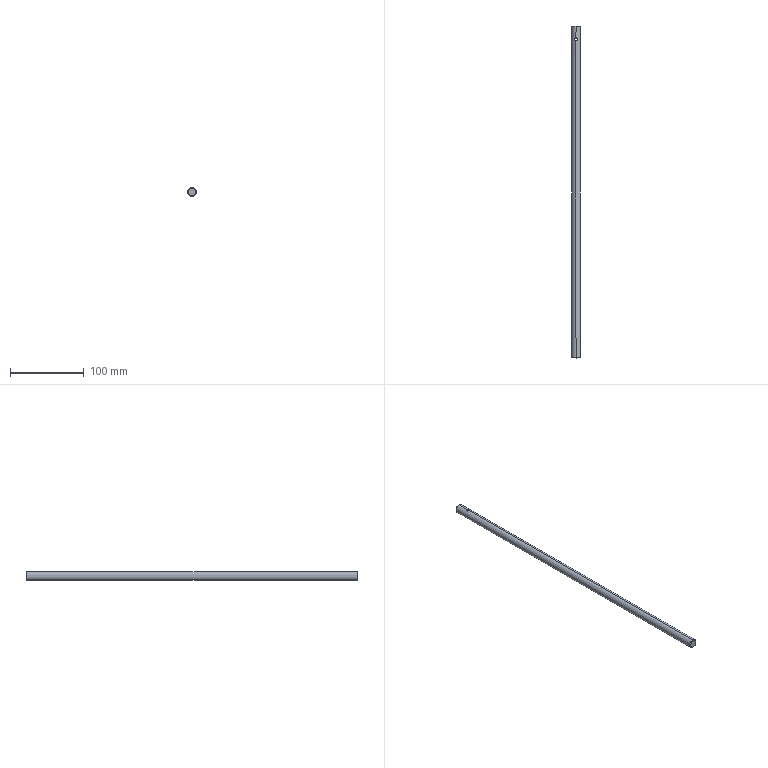Part | SolidWorks | features Chamfer 1, Extrusion 1, ICE 1 | 1 solid | 10 faces | box 12 x 450 x 12 mm | volume 50710 mm3 | cylinder 4 | cone 4 | plane 2 | commonest cylinder face diameters 4 x2 12 x2
STEP:
#1=CARTESIAN_POINT('',(-2.,207.,-5.657));
#2=VERTEX_POINT('',#1);
#3=CARTESIAN_POINT('',(0.,205.,-6.));
#4=VERTEX_POINT('',#3);
#5=CARTESIAN_POINT('',(-2.,207.,-5.657));
#6=CARTESIAN_POINT('',(-2.,206.869,-5.657));
#7=CARTESIAN_POINT('',(-1.987,206.735,-5.662));
#8=CARTESIAN_POINT('',(-1.935,206.478,-5.679));
#9=CARTESIAN_POINT('',(-1.897,206.353,-5.693));
#10=CARTESIAN_POINT('',(-1.796,206.109,-5.725));
#11=CARTESIAN_POINT('',(-1.734,205.994,-5.745));
#12=CARTESIAN_POINT('',(-1.589,205.779,-5.786));
#13=CARTESIAN_POINT('',(-1.505,205.677,-5.809));
#14=CARTESIAN_POINT('',(-1.321,205.493,-5.853));
#15=CARTESIAN_POINT('',(-1.221,205.411,-5.875));
#16=CARTESIAN_POINT('',(-1.005,205.266,-5.916));
#17=CARTESIAN_POINT('',(-0.8882,205.203,-5.935));
#18=CARTESIAN_POINT('',(-0.6474,205.103,-5.966));
#19=CARTESIAN_POINT('',(-0.5226,205.065,-5.979));
#20=CARTESIAN_POINT('',(-0.2637,205.013,-5.996));
#21=CARTESIAN_POINT('',(-0.1311,205.,-6.));
#22=CARTESIAN_POINT('',(0.,205.,-6.));
#23=B_SPLINE_CURVE_WITH_KNOTS('',3,(#5,#6,#7,#8,#9,#10,#11,#12,#13,#14,#15,#16,#17,#18,#19,#20,#21,#22),.UNSPECIFIED.,.F.,.F.,(4,2,2,2,2,2,2,2,4),(0.00315,0.003544,0.003937,0.004331,0.004724,0.005118,0.005511,0.005905,0.006298),.UNSPECIFIED.);
#24=EDGE_CURVE('',#2,#4,#23,.T.);
#25=ORIENTED_EDGE('',*,*,#24,.F.);
#26=CARTESIAN_POINT('',(-2.,207.,5.657));
#27=VERTEX_POINT('',#26);
#28=CARTESIAN_POINT('',(-2.,207.,-6.));
#29=DIRECTION('',(0.,0.,1.));
#30=VECTOR('',#29,1000.);
#31=LINE('',#28,#30);
#32=EDGE_CURVE('',#2,#27,#31,.T.);
#33=ORIENTED_EDGE('',*,*,#32,.T.);
#34=CARTESIAN_POINT('',(0.,205.,6.));
#35=VERTEX_POINT('',#34);
#36=CARTESIAN_POINT('',(0.,205.,6.));
#37=CARTESIAN_POINT('',(-0.1315,205.,6.));
#38=CARTESIAN_POINT('',(-0.2651,205.013,5.996));
#39=CARTESIAN_POINT('',(-0.5223,205.065,5.979));
#40=CARTESIAN_POINT('',(-0.6475,205.103,5.966));
#41=CARTESIAN_POINT('',(-0.8909,205.205,5.935));
#42=CARTESIAN_POINT('',(-1.006,205.267,5.916));
#43=CARTESIAN_POINT('',(-1.222,205.411,5.875));
#44=CARTESIAN_POINT('',(-1.324,205.495,5.853));
#45=CARTESIAN_POINT('',(-1.507,205.679,5.808));
#46=CARTESIAN_POINT('',(-1.589,205.779,5.786));
#47=CARTESIAN_POINT('',(-1.734,205.995,5.744));
#48=CARTESIAN_POINT('',(-1.797,206.112,5.725));
#49=CARTESIAN_POINT('',(-1.897,206.353,5.693));
#50=CARTESIAN_POINT('',(-1.935,206.477,5.679));
#51=CARTESIAN_POINT('',(-1.987,206.736,5.662));
#52=CARTESIAN_POINT('',(-2.,206.869,5.657));
#53=CARTESIAN_POINT('',(-2.,207.,5.657));
#54=B_SPLINE_CURVE_WITH_KNOTS('',3,(#36,#37,#38,#39,#40,#41,#42,#43,#44,#45,#46,#47,#48,#49,#50,#51,#52,#53),.UNSPECIFIED.,.F.,.F.,(4,2,2,2,2,2,2,2,4),(0.00315,0.003544,0.003937,0.004331,0.004724,0.005118,0.005511,0.005905,0.006298),.UNSPECIFIED.);
#55=EDGE_CURVE('',#35,#27,#54,.T.);
#56=ORIENTED_EDGE('',*,*,#55,.F.);
#57=CARTESIAN_POINT('',(2.,207.,5.657));
#58=VERTEX_POINT('',#57);
#59=CARTESIAN_POINT('',(2.,207.,5.657));
#60=CARTESIAN_POINT('',(2.,206.867,5.657));
#61=CARTESIAN_POINT('',(1.987,206.736,5.662));
#62=CARTESIAN_POINT('',(1.935,206.479,5.679));
#63=CARTESIAN_POINT('',(1.896,206.351,5.693));
#64=CARTESIAN_POINT('',(1.796,206.11,5.725));
#65=CARTESIAN_POINT('',(1.734,205.995,5.744));
#66=CARTESIAN_POINT('',(1.589,205.779,5.786));
#67=CARTESIAN_POINT('',(1.505,205.677,5.809));
#68=CARTESIAN_POINT('',(1.23,205.402,5.876));
#69=CARTESIAN_POINT('',(1.009,205.253,5.92));
#70=CARTESIAN_POINT('',(0.648,205.103,5.966));
#71=CARTESIAN_POINT('',(0.5209,205.065,5.979));
#72=CARTESIAN_POINT('',(0.2621,205.013,5.996));
#73=CARTESIAN_POINT('',(0.1316,205.,6.));
#74=CARTESIAN_POINT('',(0.,205.,6.));
#75=B_SPLINE_CURVE_WITH_KNOTS('',3,(#59,#60,#61,#62,#63,#64,#65,#66,#67,#68,#69,#70,#71,#72,#73,#74),.UNSPECIFIED.,.F.,.F.,(4,2,2,2,2,2,2,4),(0.,0.0003937,0.0007875,0.001181,0.001575,0.002362,0.002756,0.00315),.UNSPECIFIED.);
#76=EDGE_CURVE('',#58,#35,#75,.T.);
#77=ORIENTED_EDGE('',*,*,#76,.F.);
#78=CARTESIAN_POINT('',(2.,207.,-5.657));
#79=VERTEX_POINT('',#78);
#80=CARTESIAN_POINT('',(2.,207.,-6.));
#81=DIRECTION('',(0.,0.,1.));
#82=VECTOR('',#81,1000.);
#83=LINE('',#80,#82);
#84=EDGE_CURVE('',#79,#58,#83,.T.);
#85=ORIENTED_EDGE('',*,*,#84,.F.);
#86=CARTESIAN_POINT('',(0.,205.,-6.));
#87=CARTESIAN_POINT('',(0.2623,205.,-6.));
#88=CARTESIAN_POINT('',(0.5271,205.053,-5.982));
#89=CARTESIAN_POINT('',(0.889,205.204,-5.935));
#90=CARTESIAN_POINT('',(1.006,205.267,-5.916));
#91=CARTESIAN_POINT('',(1.222,205.411,-5.875));
#92=CARTESIAN_POINT('',(1.322,205.494,-5.853));
#93=CARTESIAN_POINT('',(1.599,205.771,-5.786));
#94=CARTESIAN_POINT('',(1.745,205.989,-5.741));
#95=CARTESIAN_POINT('',(1.897,206.353,-5.692));
#96=CARTESIAN_POINT('',(1.935,206.478,-5.679));
#97=CARTESIAN_POINT('',(1.987,206.735,-5.662));
#98=CARTESIAN_POINT('',(2.,206.868,-5.657));
#99=CARTESIAN_POINT('',(2.,207.,-5.657));
#100=B_SPLINE_CURVE_WITH_KNOTS('',3,(#86,#87,#88,#89,#90,#91,#92,#93,#94,#95,#96,#97,#98,#99),.UNSPECIFIED.,.F.,.F.,(4,2,2,2,2,2,4),(0.006298,0.007085,0.007479,0.007872,0.008659,0.009053,0.009446),.UNSPECIFIED.);
#101=EDGE_CURVE('',#4,#79,#100,.T.);
#102=ORIENTED_EDGE('',*,*,#101,.F.);
#103=EDGE_LOOP('',(#25,#33,#56,#77,#85,#102));
#104=FACE_OUTER_BOUND('',#103,.T.);
#105=CARTESIAN_POINT('',(0.,207.,-6.));
#106=DIRECTION('',(0.,0.,1.));
#107=DIRECTION('',(1.,0.,0.));
#108=AXIS2_PLACEMENT_3D('',#105,#106,#107);
#109=CYLINDRICAL_SURFACE('',#108,2.);
#110=ADVANCED_FACE('',(#104),#109,.F.);
#111=CARTESIAN_POINT('',(0.,225.,5.));
#112=VERTEX_POINT('',#111);
#113=CARTESIAN_POINT('',(0.,225.,-5.));
#114=VERTEX_POINT('',#113);
#115=CARTESIAN_POINT('',(0.,225.,0.));
#116=DIRECTION('',(0.,1.,0.));
#117=DIRECTION('',(0.,0.,1.));
#118=AXIS2_PLACEMENT_3D('',#115,#116,#117);
#119=CIRCLE('',#118,5.);
#120=EDGE_CURVE('',#112,#114,#119,.T.);
#121=ORIENTED_EDGE('',*,*,#120,.F.);
#122=CARTESIAN_POINT('',(0.,224.,6.));
#123=VERTEX_POINT('',#122);
#124=CARTESIAN_POINT('',(0.,225.,5.));
#125=DIRECTION('',(0.,-0.7071,0.7071));
#126=VECTOR('',#125,1000.);
#127=LINE('',#124,#126);
#128=EDGE_CURVE('',#112,#123,#127,.T.);
#129=ORIENTED_EDGE('',*,*,#128,.T.);
#130=CARTESIAN_POINT('',(0.,224.,-6.));
#131=VERTEX_POINT('',#130);
#132=CARTESIAN_POINT('',(0.,224.,0.));
#133=DIRECTION('',(0.,-1.,0.));
#134=DIRECTION('',(0.,0.,1.));
#135=AXIS2_PLACEMENT_3D('',#132,#133,#134);
#136=CIRCLE('',#135,6.);
#137=EDGE_CURVE('',#131,#123,#136,.T.);
#138=ORIENTED_EDGE('',*,*,#137,.F.);
#139=CARTESIAN_POINT('',(0.,225.,-5.));
#140=DIRECTION('',(0.,-0.7071,-0.7071));
#141=VECTOR('',#140,1000.);
#142=LINE('',#139,#141);
#143=EDGE_CURVE('',#114,#131,#142,.T.);
#144=ORIENTED_EDGE('',*,*,#143,.F.);
#145=EDGE_LOOP('',(#121,#129,#138,#144));
#146=FACE_OUTER_BOUND('',#145,.T.);
#147=CARTESIAN_POINT('',(0.,225.,0.));
#148=DIRECTION('',(0.,-1.,0.));
#149=DIRECTION('',(0.,0.,-1.));
#150=AXIS2_PLACEMENT_3D('',#147,#148,#149);
#151=CONICAL_SURFACE('',#150,5.,0.7854);
#152=ADVANCED_FACE('',(#146),#151,.T.);
#153=CARTESIAN_POINT('',(0.,-225.,-5.));
#154=VERTEX_POINT('',#153);
#155=CARTESIAN_POINT('',(0.,-225.,5.));
#156=VERTEX_POINT('',#155);
#157=CARTESIAN_POINT('',(0.,-225.,0.));
#158=DIRECTION('',(0.,-1.,0.));
#159=DIRECTION('',(0.,0.,1.));
#160=AXIS2_PLACEMENT_3D('',#157,#158,#159);
#161=CIRCLE('',#160,5.);
#162=EDGE_CURVE('',#154,#156,#161,.T.);
#163=ORIENTED_EDGE('',*,*,#162,.F.);
#164=CARTESIAN_POINT('',(0.,-224.,-6.));
#165=VERTEX_POINT('',#164);
#166=CARTESIAN_POINT('',(0.,-224.,-6.));
#167=DIRECTION('',(0.,0.7071,-0.7071));
#168=VECTOR('',#167,1000.);
#169=LINE('',#166,#168);
#170=EDGE_CURVE('',#154,#165,#169,.T.);
#171=ORIENTED_EDGE('',*,*,#170,.T.);
#172=CARTESIAN_POINT('',(0.,-224.,6.));
#173=VERTEX_POINT('',#172);
#174=CARTESIAN_POINT('',(0.,-224.,0.));
#175=DIRECTION('',(0.,1.,0.));
#176=DIRECTION('',(0.,0.,1.));
#177=AXIS2_PLACEMENT_3D('',#174,#175,#176);
#178=CIRCLE('',#177,6.);
#179=EDGE_CURVE('',#173,#165,#178,.T.);
#180=ORIENTED_EDGE('',*,*,#179,.F.);
#181=CARTESIAN_POINT('',(0.,-224.,6.));
#182=DIRECTION('',(0.,0.7071,0.7071));
#183=VECTOR('',#182,1000.);
#184=LINE('',#181,#183);
#185=EDGE_CURVE('',#156,#173,#184,.T.);
#186=ORIENTED_EDGE('',*,*,#185,.F.);
#187=EDGE_LOOP('',(#163,#171,#180,#186));
#188=FACE_OUTER_BOUND('',#187,.T.);
#189=CARTESIAN_POINT('',(0.,-224.,0.));
#190=DIRECTION('',(0.,1.,0.));
#191=DIRECTION('',(0.,0.,1.));
#192=AXIS2_PLACEMENT_3D('',#189,#190,#191);
#193=CONICAL_SURFACE('',#192,6.,0.7854);
#194=ADVANCED_FACE('',(#188),#193,.T.);
#195=ORIENTED_EDGE('',*,*,#137,.T.);
#196=CARTESIAN_POINT('',(0.,209.,6.));
#197=VERTEX_POINT('',#196);
#198=CARTESIAN_POINT('',(0.,225.,6.));
#199=DIRECTION('',(0.,-1.,0.));
#200=VECTOR('',#199,1000.);
#201=LINE('',#198,#200);
#202=EDGE_CURVE('',#123,#197,#201,.T.);
#203=ORIENTED_EDGE('',*,*,#202,.T.);
#204=CARTESIAN_POINT('',(0.,209.,6.));
#205=CARTESIAN_POINT('',(0.1318,209.,6.));
#206=CARTESIAN_POINT('',(0.2623,208.987,5.996));
#207=CARTESIAN_POINT('',(0.5209,208.935,5.979));
#208=CARTESIAN_POINT('',(0.6482,208.897,5.966));
#209=CARTESIAN_POINT('',(1.01,208.746,5.919));
#210=CARTESIAN_POINT('',(1.231,208.597,5.875));
#211=CARTESIAN_POINT('',(1.506,208.323,5.809));
#212=CARTESIAN_POINT('',(1.59,208.22,5.786));
#213=CARTESIAN_POINT('',(1.734,208.004,5.744));
#214=CARTESIAN_POINT('',(1.796,207.89,5.725));
#215=CARTESIAN_POINT('',(1.897,207.648,5.693));
#216=CARTESIAN_POINT('',(1.935,207.521,5.679));
#217=CARTESIAN_POINT('',(1.987,207.264,5.662));
#218=CARTESIAN_POINT('',(2.,207.133,5.657));
#219=CARTESIAN_POINT('',(2.,207.,5.657));
#220=B_SPLINE_CURVE_WITH_KNOTS('',3,(#204,#205,#206,#207,#208,#209,#210,#211,#212,#213,#214,#215,#216,#217,#218,#219),.UNSPECIFIED.,.F.,.F.,(4,2,2,2,2,2,2,4),(0.009446,0.00984,0.01023,0.01102,0.01141,0.01181,0.0122,0.01259),.UNSPECIFIED.);
#221=EDGE_CURVE('',#197,#58,#220,.T.);
#222=ORIENTED_EDGE('',*,*,#221,.T.);
#223=ORIENTED_EDGE('',*,*,#76,.T.);
#224=CARTESIAN_POINT('',(0.,225.,6.));
#225=DIRECTION('',(0.,-1.,0.));
#226=VECTOR('',#225,1000.);
#227=LINE('',#224,#226);
#228=EDGE_CURVE('',#35,#173,#227,.T.);
#229=ORIENTED_EDGE('',*,*,#228,.T.);
#230=ORIENTED_EDGE('',*,*,#179,.T.);
#231=CARTESIAN_POINT('',(0.,225.,-6.));
#232=DIRECTION('',(0.,-1.,0.));
#233=VECTOR('',#232,1000.);
#234=LINE('',#231,#233);
#235=EDGE_CURVE('',#4,#165,#234,.T.);
#236=ORIENTED_EDGE('',*,*,#235,.F.);
#237=ORIENTED_EDGE('',*,*,#101,.T.);
#238=CARTESIAN_POINT('',(0.,209.,-6.));
#239=VERTEX_POINT('',#238);
#240=CARTESIAN_POINT('',(2.,207.,-5.657));
#241=CARTESIAN_POINT('',(2.,207.132,-5.657));
#242=CARTESIAN_POINT('',(1.987,207.262,-5.661));
#243=CARTESIAN_POINT('',(1.935,207.521,-5.679));
#244=CARTESIAN_POINT('',(1.897,207.648,-5.693));
#245=CARTESIAN_POINT('',(1.746,208.009,-5.741));
#246=CARTESIAN_POINT('',(1.598,208.231,-5.786));
#247=CARTESIAN_POINT('',(1.323,208.506,-5.853));
#248=CARTESIAN_POINT('',(1.221,208.59,-5.876));
#249=CARTESIAN_POINT('',(1.005,208.734,-5.916));
#250=CARTESIAN_POINT('',(0.8903,208.796,-5.935));
#251=CARTESIAN_POINT('',(0.6484,208.896,-5.966));
#252=CARTESIAN_POINT('',(0.5209,208.935,-5.979));
#253=CARTESIAN_POINT('',(0.264,208.987,-5.996));
#254=CARTESIAN_POINT('',(0.1331,209.,-6.));
#255=CARTESIAN_POINT('',(0.,209.,-6.));
#256=B_SPLINE_CURVE_WITH_KNOTS('',3,(#240,#241,#242,#243,#244,#245,#246,#247,#248,#249,#250,#251,#252,#253,#254,#255),.UNSPECIFIED.,.F.,.F.,(4,2,2,2,2,2,2,4),(0.009446,0.00984,0.01023,0.01102,0.01141,0.01181,0.0122,0.0126),.UNSPECIFIED.);
#257=EDGE_CURVE('',#79,#239,#256,.T.);
#258=ORIENTED_EDGE('',*,*,#257,.T.);
#259=CARTESIAN_POINT('',(0.,225.,-6.));
#260=DIRECTION('',(0.,-1.,0.));
#261=VECTOR('',#260,1000.);
#262=LINE('',#259,#261);
#263=EDGE_CURVE('',#131,#239,#262,.T.);
#264=ORIENTED_EDGE('',*,*,#263,.F.);
#265=EDGE_LOOP('',(#195,#203,#222,#223,#229,#230,#236,#237,#258,#264));
#266=FACE_OUTER_BOUND('',#265,.T.);
#267=CARTESIAN_POINT('',(0.,225.,0.));
#268=DIRECTION('',(0.,-1.,0.));
#269=DIRECTION('',(0.,0.,-1.));
#270=AXIS2_PLACEMENT_3D('',#267,#268,#269);
#271=CYLINDRICAL_SURFACE('',#270,6.);
#272=ADVANCED_FACE('',(#266),#271,.T.);
#273=ORIENTED_EDGE('',*,*,#202,.F.);
#274=CARTESIAN_POINT('',(0.,224.,0.));
#275=DIRECTION('',(0.,-1.,0.));
#276=DIRECTION('',(0.,0.,1.));
#277=AXIS2_PLACEMENT_3D('',#274,#275,#276);
#278=CIRCLE('',#277,6.);
#279=EDGE_CURVE('',#123,#131,#278,.T.);
#280=ORIENTED_EDGE('',*,*,#279,.T.);
#281=ORIENTED_EDGE('',*,*,#263,.T.);
#282=CARTESIAN_POINT('',(0.,209.,-6.));
#283=CARTESIAN_POINT('',(-0.1332,209.,-6.));
#284=CARTESIAN_POINT('',(-0.264,208.987,-5.996));
#285=CARTESIAN_POINT('',(-0.5211,208.935,-5.979));
#286=CARTESIAN_POINT('',(-0.6487,208.896,-5.966));
#287=CARTESIAN_POINT('',(-0.8906,208.796,-5.935));
#288=CARTESIAN_POINT('',(-1.005,208.734,-5.916));
#289=CARTESIAN_POINT('',(-1.222,208.589,-5.875));
#290=CARTESIAN_POINT('',(-1.324,208.505,-5.853));
#291=CARTESIAN_POINT('',(-1.598,208.23,-5.786));
#292=CARTESIAN_POINT('',(-1.747,208.008,-5.741));
#293=CARTESIAN_POINT('',(-1.897,207.648,-5.693));
#294=CARTESIAN_POINT('',(-1.936,207.521,-5.679));
#295=CARTESIAN_POINT('',(-1.987,207.262,-5.661));
#296=CARTESIAN_POINT('',(-2.,207.132,-5.657));
#297=CARTESIAN_POINT('',(-2.,207.,-5.657));
#298=B_SPLINE_CURVE_WITH_KNOTS('',3,(#282,#283,#284,#285,#286,#287,#288,#289,#290,#291,#292,#293,#294,#295,#296,#297),.UNSPECIFIED.,.F.,.F.,(4,2,2,2,2,2,2,4),(0.,0.0003938,0.0007875,0.001181,0.001575,0.002363,0.002756,0.00315),.UNSPECIFIED.);
#299=EDGE_CURVE('',#239,#2,#298,.T.);
#300=ORIENTED_EDGE('',*,*,#299,.T.);
#301=ORIENTED_EDGE('',*,*,#24,.T.);
#302=ORIENTED_EDGE('',*,*,#235,.T.);
#303=CARTESIAN_POINT('',(0.,-224.,0.));
#304=DIRECTION('',(0.,1.,0.));
#305=DIRECTION('',(0.,0.,1.));
#306=AXIS2_PLACEMENT_3D('',#303,#304,#305);
#307=CIRCLE('',#306,6.);
#308=EDGE_CURVE('',#165,#173,#307,.T.);
#309=ORIENTED_EDGE('',*,*,#308,.T.);
#310=ORIENTED_EDGE('',*,*,#228,.F.);
#311=ORIENTED_EDGE('',*,*,#55,.T.);
#312=CARTESIAN_POINT('',(-2.,207.,5.657));
#313=CARTESIAN_POINT('',(-2.,207.262,5.657));
#314=CARTESIAN_POINT('',(-1.947,207.527,5.676));
#315=CARTESIAN_POINT('',(-1.796,207.889,5.725));
#316=CARTESIAN_POINT('',(-1.734,208.006,5.745));
#317=CARTESIAN_POINT('',(-1.589,208.222,5.786));
#318=CARTESIAN_POINT('',(-1.507,208.322,5.809));
#319=CARTESIAN_POINT('',(-1.23,208.599,5.876));
#320=CARTESIAN_POINT('',(-1.012,208.745,5.919));
#321=CARTESIAN_POINT('',(-0.6469,208.897,5.966));
#322=CARTESIAN_POINT('',(-0.5219,208.935,5.979));
#323=CARTESIAN_POINT('',(-0.2652,208.987,5.996));
#324=CARTESIAN_POINT('',(-0.1318,209.,6.));
#325=CARTESIAN_POINT('',(0.,209.,6.));
#326=B_SPLINE_CURVE_WITH_KNOTS('',3,(#312,#313,#314,#315,#316,#317,#318,#319,#320,#321,#322,#323,#324,#325),.UNSPECIFIED.,.F.,.F.,(4,2,2,2,2,2,4),(0.006298,0.007085,0.007479,0.007872,0.008659,0.009053,0.009446),.UNSPECIFIED.);
#327=EDGE_CURVE('',#27,#197,#326,.T.);
#328=ORIENTED_EDGE('',*,*,#327,.T.);
#329=EDGE_LOOP('',(#273,#280,#281,#300,#301,#302,#309,#310,#311,#328));
#330=FACE_OUTER_BOUND('',#329,.T.);
#331=CARTESIAN_POINT('',(0.,225.,0.));
#332=DIRECTION('',(0.,-1.,0.));
#333=DIRECTION('',(0.,0.,-1.));
#334=AXIS2_PLACEMENT_3D('',#331,#332,#333);
#335=CYLINDRICAL_SURFACE('',#334,6.);
#336=ADVANCED_FACE('',(#330),#335,.T.);
#337=CARTESIAN_POINT('',(0.,225.,0.));
#338=DIRECTION('',(0.,1.,0.));
#339=DIRECTION('',(0.,0.,1.));
#340=AXIS2_PLACEMENT_3D('',#337,#338,#339);
#341=CIRCLE('',#340,5.);
#342=EDGE_CURVE('',#114,#112,#341,.T.);
#343=ORIENTED_EDGE('',*,*,#342,.T.);
#344=ORIENTED_EDGE('',*,*,#120,.T.);
#345=EDGE_LOOP('',(#343,#344));
#346=FACE_OUTER_BOUND('',#345,.T.);
#347=CARTESIAN_POINT('',(0.,225.,0.));
#348=DIRECTION('',(0.,1.,0.));
#349=DIRECTION('',(0.,0.,1.));
#350=AXIS2_PLACEMENT_3D('',#347,#348,#349);
#351=PLANE('',#350);
#352=ADVANCED_FACE('',(#346),#351,.T.);
#353=CARTESIAN_POINT('',(0.,-225.,0.));
#354=DIRECTION('',(0.,-1.,0.));
#355=DIRECTION('',(0.,0.,1.));
#356=AXIS2_PLACEMENT_3D('',#353,#354,#355);
#357=CIRCLE('',#356,5.);
#358=EDGE_CURVE('',#156,#154,#357,.T.);
#359=ORIENTED_EDGE('',*,*,#358,.T.);
#360=ORIENTED_EDGE('',*,*,#162,.T.);
#361=EDGE_LOOP('',(#359,#360));
#362=FACE_OUTER_BOUND('',#361,.T.);
#363=CARTESIAN_POINT('',(0.,-225.,0.));
#364=DIRECTION('',(0.,1.,0.));
#365=DIRECTION('',(0.,0.,1.));
#366=AXIS2_PLACEMENT_3D('',#363,#364,#365);
#367=PLANE('',#366);
#368=ADVANCED_FACE('',(#362),#367,.F.);
#369=ORIENTED_EDGE('',*,*,#170,.F.);
#370=ORIENTED_EDGE('',*,*,#358,.F.);
#371=ORIENTED_EDGE('',*,*,#185,.T.);
#372=ORIENTED_EDGE('',*,*,#308,.F.);
#373=EDGE_LOOP('',(#369,#370,#371,#372));
#374=FACE_OUTER_BOUND('',#373,.T.);
#375=CARTESIAN_POINT('',(0.,-224.,0.));
#376=DIRECTION('',(0.,1.,0.));
#377=DIRECTION('',(0.,0.,1.));
#378=AXIS2_PLACEMENT_3D('',#375,#376,#377);
#379=CONICAL_SURFACE('',#378,6.,0.7854);
#380=ADVANCED_FACE('',(#374),#379,.T.);
#381=ORIENTED_EDGE('',*,*,#128,.F.);
#382=ORIENTED_EDGE('',*,*,#342,.F.);
#383=ORIENTED_EDGE('',*,*,#143,.T.);
#384=ORIENTED_EDGE('',*,*,#279,.F.);
#385=EDGE_LOOP('',(#381,#382,#383,#384));
#386=FACE_OUTER_BOUND('',#385,.T.);
#387=CARTESIAN_POINT('',(0.,225.,0.));
#388=DIRECTION('',(0.,-1.,0.));
#389=DIRECTION('',(0.,0.,-1.));
#390=AXIS2_PLACEMENT_3D('',#387,#388,#389);
#391=CONICAL_SURFACE('',#390,5.,0.7854);
#392=ADVANCED_FACE('',(#386),#391,.T.);
#393=ORIENTED_EDGE('',*,*,#32,.F.);
#394=ORIENTED_EDGE('',*,*,#299,.F.);
#395=ORIENTED_EDGE('',*,*,#257,.F.);
#396=ORIENTED_EDGE('',*,*,#84,.T.);
#397=ORIENTED_EDGE('',*,*,#221,.F.);
#398=ORIENTED_EDGE('',*,*,#327,.F.);
#399=EDGE_LOOP('',(#393,#394,#395,#396,#397,#398));
#400=FACE_OUTER_BOUND('',#399,.T.);
#401=CARTESIAN_POINT('',(0.,207.,-6.));
#402=DIRECTION('',(0.,0.,1.));
#403=DIRECTION('',(1.,0.,0.));
#404=AXIS2_PLACEMENT_3D('',#401,#402,#403);
#405=CYLINDRICAL_SURFACE('',#404,2.);
#406=ADVANCED_FACE('',(#400),#405,.F.);
#407=CLOSED_SHELL('',(#110,#152,#194,#272,#336,#352,#368,#380,#392,#406));
#408=MANIFOLD_SOLID_BREP('',#407);
#409=CARTESIAN_POINT('',(0.,0.,0.));
#410=DIRECTION('',(0.,0.,1.));
#411=DIRECTION('',(1.,0.,0.));
#412=AXIS2_PLACEMENT_3D('',#409,#410,#411);
#413=(LENGTH_UNIT()NAMED_UNIT(*)SI_UNIT(.MILLI.,.METRE.));
#414=UNCERTAINTY_MEASURE_WITH_UNIT(LENGTH_MEASURE(0.00001),#413,'','');
#415=(NAMED_UNIT(*)PLANE_ANGLE_UNIT()SI_UNIT($,.RADIAN.));
#416=(NAMED_UNIT(*)SI_UNIT($,.STERADIAN.)SOLID_ANGLE_UNIT());
#417=(GEOMETRIC_REPRESENTATION_CONTEXT(3)GLOBAL_UNCERTAINTY_ASSIGNED_CONTEXT((#414))GLOBAL_UNIT_ASSIGNED_CONTEXT((#413,#415,#416))REPRESENTATION_CONTEXT('',''));
#418=ADVANCED_BREP_SHAPE_REPRESENTATION('',(#408,#412),#417);